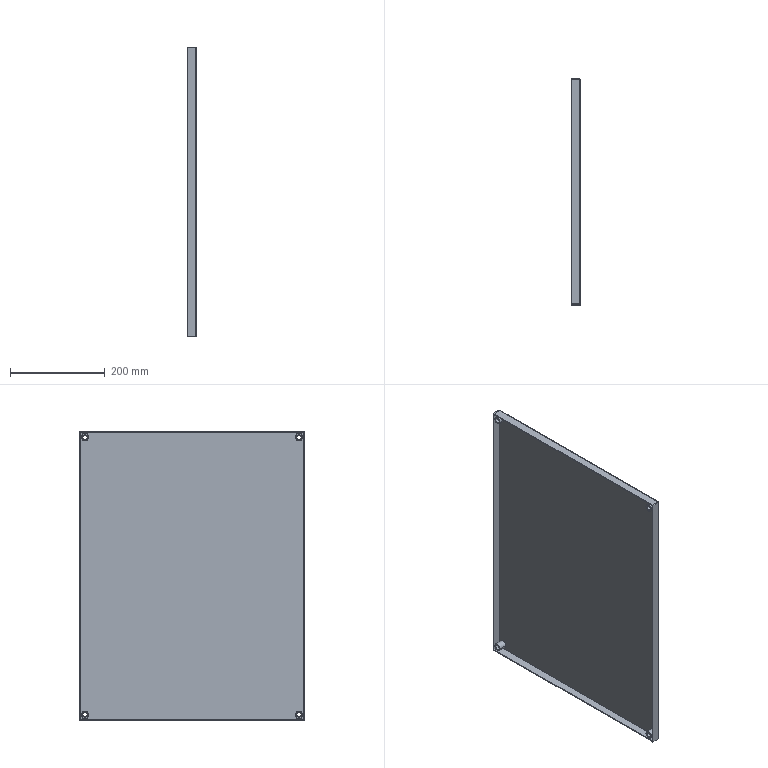Part | SolidWorks | 5 solids | 70 faces | box 19 x 477 x 612 mm | volume 663374 mm3 | plane 34 | cylinder 32 | spline 4 | commonest cylinder face diameters 9 x8 10 x8 16 x8 0.2 x4 4.2 x4